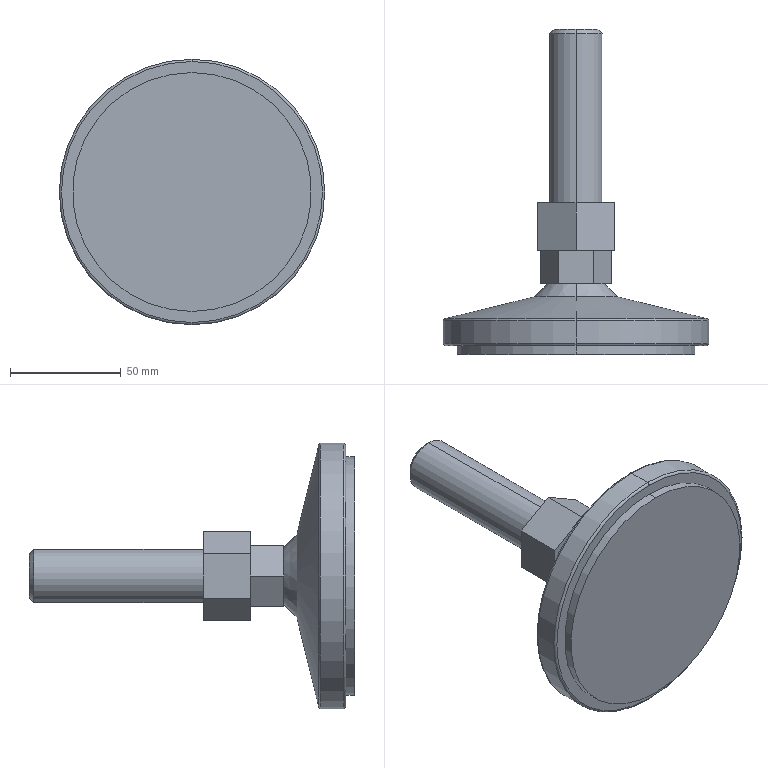Part | STEP file | 1 solid | 34 faces | box 120 x 147 x 120 mm | volume 298172 mm3 | plane 18 | cylinder 6 | cone 6 | torus 4 | commonest cylinder face diameters 24 x2 108 x2 120 x2